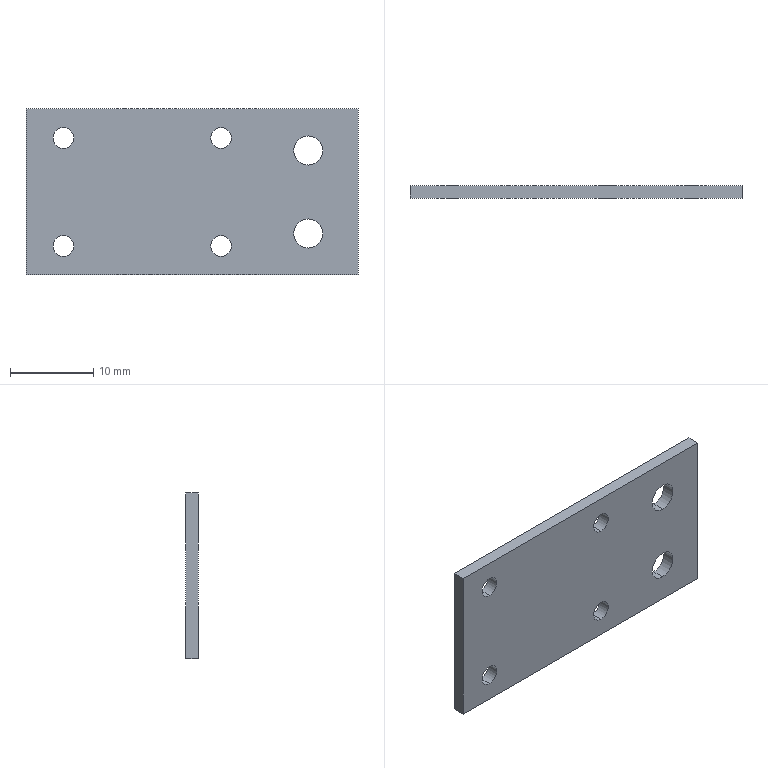Part | STEP file | 0243_224_Plate | 1 solid | 18 faces | box 40 x 1.5 x 20 mm | volume 1142 mm3 | cylinder 12 | plane 6 | commonest cylinder face diameters 2.5 x8 3.5 x4
STEP:
#1=CARTESIAN_POINT('',(0.,0.,0.));
#2=DIRECTION('',(0.,0.,1.));
#3=DIRECTION('',(1.,0.,0.));
#4=AXIS2_PLACEMENT_3D('',#1,#2,#3);
#5=CARTESIAN_POINT('',(-16.5,0.,7.75));
#6=VERTEX_POINT('',#5);
#7=CARTESIAN_POINT('',(-16.5,1.5,7.75));
#8=VERTEX_POINT('',#7);
#9=CARTESIAN_POINT('',(-16.5,1.5,7.75));
#10=DIRECTION('',(0.,1.,0.));
#11=VECTOR('',#10,1.);
#12=LINE('',#9,#11);
#13=CARTESIAN_POINT('',(-16.5,1.5,6.5));
#14=DIRECTION('',(0.,1.,0.));
#15=DIRECTION('',(0.,0.,1.));
#16=AXIS2_PLACEMENT_3D('',#13,#14,#15);
#17=CYLINDRICAL_SURFACE('',#16,1.25);
#18=CARTESIAN_POINT('',(6.283,0.));
#19=DIRECTION('',(0.,1.));
#20=VECTOR('',#19,1.);
#21=LINE('',#18,#20);
#22=(GEOMETRIC_REPRESENTATION_CONTEXT(2)PARAMETRIC_REPRESENTATION_CONTEXT()REPRESENTATION_CONTEXT('',''));
#23=DEFINITIONAL_REPRESENTATION('',(#21),#22);
#24=PCURVE('',#17,#23);
#25=CARTESIAN_POINT('',(-16.5,1.5,6.5));
#26=DIRECTION('',(0.,1.,0.));
#27=DIRECTION('',(0.,0.,1.));
#28=AXIS2_PLACEMENT_3D('',#25,#26,#27);
#29=CYLINDRICAL_SURFACE('',#28,1.25);
#30=CARTESIAN_POINT('',(0.,0.));
#31=DIRECTION('',(0.,1.));
#32=VECTOR('',#31,1.);
#33=LINE('',#30,#32);
#34=(GEOMETRIC_REPRESENTATION_CONTEXT(2)PARAMETRIC_REPRESENTATION_CONTEXT()REPRESENTATION_CONTEXT('',''));
#35=DEFINITIONAL_REPRESENTATION('',(#33),#34);
#36=PCURVE('',#29,#35);
#37=SURFACE_CURVE('',#12,(#24,#36),.PCURVE_S1.);
#38=EDGE_CURVE('',#6,#8,#37,.T.);
#39=ORIENTED_EDGE('',*,*,#38,.T.);
#40=CARTESIAN_POINT('',(-16.5,1.5,5.25));
#41=VERTEX_POINT('',#40);
#42=CARTESIAN_POINT('',(-16.5,1.5,6.5));
#43=DIRECTION('',(0.,1.,0.));
#44=DIRECTION('',(0.,0.,1.));
#45=AXIS2_PLACEMENT_3D('',#42,#43,#44);
#46=CIRCLE('',#45,1.25);
#47=CARTESIAN_POINT('',(0.,0.));
#48=DIRECTION('',(1.,0.));
#49=VECTOR('',#48,1.);
#50=LINE('',#47,#49);
#51=(GEOMETRIC_REPRESENTATION_CONTEXT(2)PARAMETRIC_REPRESENTATION_CONTEXT()REPRESENTATION_CONTEXT('',''));
#52=DEFINITIONAL_REPRESENTATION('',(#50),#51);
#53=PCURVE('',#17,#52);
#54=CARTESIAN_POINT('',(0.,1.5,-10.));
#55=DIRECTION('',(0.,1.,0.));
#56=DIRECTION('',(0.,0.,1.));
#57=AXIS2_PLACEMENT_3D('',#54,#55,#56);
#58=PLANE('',#57);
#59=CARTESIAN_POINT('',(16.5,-16.5));
#60=DIRECTION('',(1.,0.));
#61=AXIS2_PLACEMENT_2D('',#59,#60);
#62=CIRCLE('',#61,1.25);
#63=(GEOMETRIC_REPRESENTATION_CONTEXT(2)PARAMETRIC_REPRESENTATION_CONTEXT()REPRESENTATION_CONTEXT('',''));
#64=DEFINITIONAL_REPRESENTATION('',(#62),#63);
#65=PCURVE('',#58,#64);
#66=SURFACE_CURVE('',#46,(#53,#65),.PCURVE_S1.);
#67=EDGE_CURVE('',#41,#8,#66,.T.);
#68=ORIENTED_EDGE('',*,*,#67,.F.);
#69=CARTESIAN_POINT('',(-16.5,0.,5.25));
#70=VERTEX_POINT('',#69);
#71=CARTESIAN_POINT('',(-16.5,1.5,5.25));
#72=DIRECTION('',(0.,1.,0.));
#73=VECTOR('',#72,1.);
#74=LINE('',#71,#73);
#75=CARTESIAN_POINT('',(3.142,0.));
#76=DIRECTION('',(0.,1.));
#77=VECTOR('',#76,1.);
#78=LINE('',#75,#77);
#79=(GEOMETRIC_REPRESENTATION_CONTEXT(2)PARAMETRIC_REPRESENTATION_CONTEXT()REPRESENTATION_CONTEXT('',''));
#80=DEFINITIONAL_REPRESENTATION('',(#78),#79);
#81=PCURVE('',#17,#80);
#82=CARTESIAN_POINT('',(3.142,0.));
#83=DIRECTION('',(0.,1.));
#84=VECTOR('',#83,1.);
#85=LINE('',#82,#84);
#86=(GEOMETRIC_REPRESENTATION_CONTEXT(2)PARAMETRIC_REPRESENTATION_CONTEXT()REPRESENTATION_CONTEXT('',''));
#87=DEFINITIONAL_REPRESENTATION('',(#85),#86);
#88=PCURVE('',#29,#87);
#89=SURFACE_CURVE('',#74,(#81,#88),.PCURVE_S1.);
#90=EDGE_CURVE('',#70,#41,#89,.T.);
#91=ORIENTED_EDGE('',*,*,#90,.F.);
#92=CARTESIAN_POINT('',(-16.5,0.,6.5));
#93=DIRECTION('',(0.,1.,0.));
#94=DIRECTION('',(0.,0.,1.));
#95=AXIS2_PLACEMENT_3D('',#92,#93,#94);
#96=CIRCLE('',#95,1.25);
#97=CARTESIAN_POINT('',(0.,-1.5));
#98=DIRECTION('',(1.,0.));
#99=VECTOR('',#98,1.);
#100=LINE('',#97,#99);
#101=(GEOMETRIC_REPRESENTATION_CONTEXT(2)PARAMETRIC_REPRESENTATION_CONTEXT()REPRESENTATION_CONTEXT('',''));
#102=DEFINITIONAL_REPRESENTATION('',(#100),#101);
#103=PCURVE('',#17,#102);
#104=CARTESIAN_POINT('',(0.,0.,-10.));
#105=DIRECTION('',(0.,1.,0.));
#106=DIRECTION('',(0.,0.,1.));
#107=AXIS2_PLACEMENT_3D('',#104,#105,#106);
#108=PLANE('',#107);
#109=CARTESIAN_POINT('',(16.5,-16.5));
#110=DIRECTION('',(1.,0.));
#111=AXIS2_PLACEMENT_2D('',#109,#110);
#112=CIRCLE('',#111,1.25);
#113=(GEOMETRIC_REPRESENTATION_CONTEXT(2)PARAMETRIC_REPRESENTATION_CONTEXT()REPRESENTATION_CONTEXT('',''));
#114=DEFINITIONAL_REPRESENTATION('',(#112),#113);
#115=PCURVE('',#108,#114);
#116=SURFACE_CURVE('',#96,(#103,#115),.PCURVE_S1.);
#117=EDGE_CURVE('',#70,#6,#116,.T.);
#118=ORIENTED_EDGE('',*,*,#117,.T.);
#119=EDGE_LOOP('',(#39,#68,#91,#118));
#120=FACE_BOUND('',#119,.F.);
#121=ADVANCED_FACE('',(#120),#17,.F.);
#122=CARTESIAN_POINT('',(-16.5,0.,-5.25));
#123=VERTEX_POINT('',#122);
#124=CARTESIAN_POINT('',(-16.5,1.5,-5.25));
#125=VERTEX_POINT('',#124);
#126=CARTESIAN_POINT('',(-16.5,1.5,-5.25));
#127=DIRECTION('',(0.,1.,0.));
#128=VECTOR('',#127,1.);
#129=LINE('',#126,#128);
#130=CARTESIAN_POINT('',(-16.5,1.5,-6.5));
#131=DIRECTION('',(0.,1.,0.));
#132=DIRECTION('',(0.,0.,1.));
#133=AXIS2_PLACEMENT_3D('',#130,#131,#132);
#134=CYLINDRICAL_SURFACE('',#133,1.25);
#135=CARTESIAN_POINT('',(6.283,0.));
#136=DIRECTION('',(0.,1.));
#137=VECTOR('',#136,1.);
#138=LINE('',#135,#137);
#139=(GEOMETRIC_REPRESENTATION_CONTEXT(2)PARAMETRIC_REPRESENTATION_CONTEXT()REPRESENTATION_CONTEXT('',''));
#140=DEFINITIONAL_REPRESENTATION('',(#138),#139);
#141=PCURVE('',#134,#140);
#142=CARTESIAN_POINT('',(-16.5,1.5,-6.5));
#143=DIRECTION('',(0.,1.,0.));
#144=DIRECTION('',(0.,0.,1.));
#145=AXIS2_PLACEMENT_3D('',#142,#143,#144);
#146=CYLINDRICAL_SURFACE('',#145,1.25);
#147=CARTESIAN_POINT('',(0.,0.));
#148=DIRECTION('',(0.,1.));
#149=VECTOR('',#148,1.);
#150=LINE('',#147,#149);
#151=(GEOMETRIC_REPRESENTATION_CONTEXT(2)PARAMETRIC_REPRESENTATION_CONTEXT()REPRESENTATION_CONTEXT('',''));
#152=DEFINITIONAL_REPRESENTATION('',(#150),#151);
#153=PCURVE('',#146,#152);
#154=SURFACE_CURVE('',#129,(#141,#153),.PCURVE_S1.);
#155=EDGE_CURVE('',#123,#125,#154,.T.);
#156=ORIENTED_EDGE('',*,*,#155,.T.);
#157=CARTESIAN_POINT('',(-16.5,1.5,-7.75));
#158=VERTEX_POINT('',#157);
#159=CARTESIAN_POINT('',(-16.5,1.5,-6.5));
#160=DIRECTION('',(0.,1.,0.));
#161=DIRECTION('',(0.,0.,1.));
#162=AXIS2_PLACEMENT_3D('',#159,#160,#161);
#163=CIRCLE('',#162,1.25);
#164=CARTESIAN_POINT('',(0.,0.));
#165=DIRECTION('',(1.,0.));
#166=VECTOR('',#165,1.);
#167=LINE('',#164,#166);
#168=(GEOMETRIC_REPRESENTATION_CONTEXT(2)PARAMETRIC_REPRESENTATION_CONTEXT()REPRESENTATION_CONTEXT('',''));
#169=DEFINITIONAL_REPRESENTATION('',(#167),#168);
#170=PCURVE('',#134,#169);
#171=CARTESIAN_POINT('',(3.5,-16.5));
#172=DIRECTION('',(1.,0.));
#173=AXIS2_PLACEMENT_2D('',#171,#172);
#174=CIRCLE('',#173,1.25);
#175=(GEOMETRIC_REPRESENTATION_CONTEXT(2)PARAMETRIC_REPRESENTATION_CONTEXT()REPRESENTATION_CONTEXT('',''));
#176=DEFINITIONAL_REPRESENTATION('',(#174),#175);
#177=PCURVE('',#58,#176);
#178=SURFACE_CURVE('',#163,(#170,#177),.PCURVE_S1.);
#179=EDGE_CURVE('',#158,#125,#178,.T.);
#180=ORIENTED_EDGE('',*,*,#179,.F.);
#181=CARTESIAN_POINT('',(-16.5,0.,-7.75));
#182=VERTEX_POINT('',#181);
#183=CARTESIAN_POINT('',(-16.5,1.5,-7.75));
#184=DIRECTION('',(0.,1.,0.));
#185=VECTOR('',#184,1.);
#186=LINE('',#183,#185);
#187=CARTESIAN_POINT('',(3.142,0.));
#188=DIRECTION('',(0.,1.));
#189=VECTOR('',#188,1.);
#190=LINE('',#187,#189);
#191=(GEOMETRIC_REPRESENTATION_CONTEXT(2)PARAMETRIC_REPRESENTATION_CONTEXT()REPRESENTATION_CONTEXT('',''));
#192=DEFINITIONAL_REPRESENTATION('',(#190),#191);
#193=PCURVE('',#134,#192);
#194=CARTESIAN_POINT('',(3.142,0.));
#195=DIRECTION('',(0.,1.));
#196=VECTOR('',#195,1.);
#197=LINE('',#194,#196);
#198=(GEOMETRIC_REPRESENTATION_CONTEXT(2)PARAMETRIC_REPRESENTATION_CONTEXT()REPRESENTATION_CONTEXT('',''));
#199=DEFINITIONAL_REPRESENTATION('',(#197),#198);
#200=PCURVE('',#146,#199);
#201=SURFACE_CURVE('',#186,(#193,#200),.PCURVE_S1.);
#202=EDGE_CURVE('',#182,#158,#201,.T.);
#203=ORIENTED_EDGE('',*,*,#202,.F.);
#204=CARTESIAN_POINT('',(-16.5,0.,-6.5));
#205=DIRECTION('',(0.,1.,0.));
#206=DIRECTION('',(0.,0.,1.));
#207=AXIS2_PLACEMENT_3D('',#204,#205,#206);
#208=CIRCLE('',#207,1.25);
#209=CARTESIAN_POINT('',(0.,-1.5));
#210=DIRECTION('',(1.,0.));
#211=VECTOR('',#210,1.);
#212=LINE('',#209,#211);
#213=(GEOMETRIC_REPRESENTATION_CONTEXT(2)PARAMETRIC_REPRESENTATION_CONTEXT()REPRESENTATION_CONTEXT('',''));
#214=DEFINITIONAL_REPRESENTATION('',(#212),#213);
#215=PCURVE('',#134,#214);
#216=CARTESIAN_POINT('',(3.5,-16.5));
#217=DIRECTION('',(1.,0.));
#218=AXIS2_PLACEMENT_2D('',#216,#217);
#219=CIRCLE('',#218,1.25);
#220=(GEOMETRIC_REPRESENTATION_CONTEXT(2)PARAMETRIC_REPRESENTATION_CONTEXT()REPRESENTATION_CONTEXT('',''));
#221=DEFINITIONAL_REPRESENTATION('',(#219),#220);
#222=PCURVE('',#108,#221);
#223=SURFACE_CURVE('',#208,(#215,#222),.PCURVE_S1.);
#224=EDGE_CURVE('',#182,#123,#223,.T.);
#225=ORIENTED_EDGE('',*,*,#224,.T.);
#226=EDGE_LOOP('',(#156,#180,#203,#225));
#227=FACE_BOUND('',#226,.F.);
#228=ADVANCED_FACE('',(#227),#134,.F.);
#229=CARTESIAN_POINT('',(-35.5,0.,-5.25));
#230=VERTEX_POINT('',#229);
#231=CARTESIAN_POINT('',(-35.5,1.5,-5.25));
#232=VERTEX_POINT('',#231);
#233=CARTESIAN_POINT('',(-35.5,1.5,-5.25));
#234=DIRECTION('',(0.,1.,0.));
#235=VECTOR('',#234,1.);
#236=LINE('',#233,#235);
#237=CARTESIAN_POINT('',(-35.5,1.5,-6.5));
#238=DIRECTION('',(0.,1.,0.));
#239=DIRECTION('',(0.,0.,1.));
#240=AXIS2_PLACEMENT_3D('',#237,#238,#239);
#241=CYLINDRICAL_SURFACE('',#240,1.25);
#242=CARTESIAN_POINT('',(6.283,0.));
#243=DIRECTION('',(0.,1.));
#244=VECTOR('',#243,1.);
#245=LINE('',#242,#244);
#246=(GEOMETRIC_REPRESENTATION_CONTEXT(2)PARAMETRIC_REPRESENTATION_CONTEXT()REPRESENTATION_CONTEXT('',''));
#247=DEFINITIONAL_REPRESENTATION('',(#245),#246);
#248=PCURVE('',#241,#247);
#249=CARTESIAN_POINT('',(-35.5,1.5,-6.5));
#250=DIRECTION('',(0.,1.,0.));
#251=DIRECTION('',(0.,0.,1.));
#252=AXIS2_PLACEMENT_3D('',#249,#250,#251);
#253=CYLINDRICAL_SURFACE('',#252,1.25);
#254=CARTESIAN_POINT('',(0.,0.));
#255=DIRECTION('',(0.,1.));
#256=VECTOR('',#255,1.);
#257=LINE('',#254,#256);
#258=(GEOMETRIC_REPRESENTATION_CONTEXT(2)PARAMETRIC_REPRESENTATION_CONTEXT()REPRESENTATION_CONTEXT('',''));
#259=DEFINITIONAL_REPRESENTATION('',(#257),#258);
#260=PCURVE('',#253,#259);
#261=SURFACE_CURVE('',#236,(#248,#260),.PCURVE_S1.);
#262=EDGE_CURVE('',#230,#232,#261,.T.);
#263=ORIENTED_EDGE('',*,*,#262,.T.);
#264=CARTESIAN_POINT('',(-35.5,1.5,-7.75));
#265=VERTEX_POINT('',#264);
#266=CARTESIAN_POINT('',(-35.5,1.5,-6.5));
#267=DIRECTION('',(0.,1.,0.));
#268=DIRECTION('',(0.,0.,1.));
#269=AXIS2_PLACEMENT_3D('',#266,#267,#268);
#270=CIRCLE('',#269,1.25);
#271=CARTESIAN_POINT('',(0.,0.));
#272=DIRECTION('',(1.,0.));
#273=VECTOR('',#272,1.);
#274=LINE('',#271,#273);
#275=(GEOMETRIC_REPRESENTATION_CONTEXT(2)PARAMETRIC_REPRESENTATION_CONTEXT()REPRESENTATION_CONTEXT('',''));
#276=DEFINITIONAL_REPRESENTATION('',(#274),#275);
#277=PCURVE('',#241,#276);
#278=CARTESIAN_POINT('',(3.5,-35.5));
#279=DIRECTION('',(1.,0.));
#280=AXIS2_PLACEMENT_2D('',#278,#279);
#281=CIRCLE('',#280,1.25);
#282=(GEOMETRIC_REPRESENTATION_CONTEXT(2)PARAMETRIC_REPRESENTATION_CONTEXT()REPRESENTATION_CONTEXT('',''));
#283=DEFINITIONAL_REPRESENTATION('',(#281),#282);
#284=PCURVE('',#58,#283);
#285=SURFACE_CURVE('',#270,(#277,#284),.PCURVE_S1.);
#286=EDGE_CURVE('',#265,#232,#285,.T.);
#287=ORIENTED_EDGE('',*,*,#286,.F.);
#288=CARTESIAN_POINT('',(-35.5,0.,-7.75));
#289=VERTEX_POINT('',#288);
#290=CARTESIAN_POINT('',(-35.5,1.5,-7.75));
#291=DIRECTION('',(0.,1.,0.));
#292=VECTOR('',#291,1.);
#293=LINE('',#290,#292);
#294=CARTESIAN_POINT('',(3.142,0.));
#295=DIRECTION('',(0.,1.));
#296=VECTOR('',#295,1.);
#297=LINE('',#294,#296);
#298=(GEOMETRIC_REPRESENTATION_CONTEXT(2)PARAMETRIC_REPRESENTATION_CONTEXT()REPRESENTATION_CONTEXT('',''));
#299=DEFINITIONAL_REPRESENTATION('',(#297),#298);
#300=PCURVE('',#241,#299);
#301=CARTESIAN_POINT('',(3.142,0.));
#302=DIRECTION('',(0.,1.));
#303=VECTOR('',#302,1.);
#304=LINE('',#301,#303);
#305=(GEOMETRIC_REPRESENTATION_CONTEXT(2)PARAMETRIC_REPRESENTATION_CONTEXT()REPRESENTATION_CONTEXT('',''));
#306=DEFINITIONAL_REPRESENTATION('',(#304),#305);
#307=PCURVE('',#253,#306);
#308=SURFACE_CURVE('',#293,(#300,#307),.PCURVE_S1.);
#309=EDGE_CURVE('',#289,#265,#308,.T.);
#310=ORIENTED_EDGE('',*,*,#309,.F.);
#311=CARTESIAN_POINT('',(-35.5,0.,-6.5));
#312=DIRECTION('',(0.,1.,0.));
#313=DIRECTION('',(0.,0.,1.));
#314=AXIS2_PLACEMENT_3D('',#311,#312,#313);
#315=CIRCLE('',#314,1.25);
#316=CARTESIAN_POINT('',(0.,-1.5));
#317=DIRECTION('',(1.,0.));
#318=VECTOR('',#317,1.);
#319=LINE('',#316,#318);
#320=(GEOMETRIC_REPRESENTATION_CONTEXT(2)PARAMETRIC_REPRESENTATION_CONTEXT()REPRESENTATION_CONTEXT('',''));
#321=DEFINITIONAL_REPRESENTATION('',(#319),#320);
#322=PCURVE('',#241,#321);
#323=CARTESIAN_POINT('',(3.5,-35.5));
#324=DIRECTION('',(1.,0.));
#325=AXIS2_PLACEMENT_2D('',#323,#324);
#326=CIRCLE('',#325,1.25);
#327=(GEOMETRIC_REPRESENTATION_CONTEXT(2)PARAMETRIC_REPRESENTATION_CONTEXT()REPRESENTATION_CONTEXT('',''));
#328=DEFINITIONAL_REPRESENTATION('',(#326),#327);
#329=PCURVE('',#108,#328);
#330=SURFACE_CURVE('',#315,(#322,#329),.PCURVE_S1.);
#331=EDGE_CURVE('',#289,#230,#330,.T.);
#332=ORIENTED_EDGE('',*,*,#331,.T.);
#333=EDGE_LOOP('',(#263,#287,#310,#332));
#334=FACE_BOUND('',#333,.F.);
#335=ADVANCED_FACE('',(#334),#241,.F.);
#336=CARTESIAN_POINT('',(-35.5,0.,7.75));
#337=VERTEX_POINT('',#336);
#338=CARTESIAN_POINT('',(-35.5,1.5,7.75));
#339=VERTEX_POINT('',#338);
#340=CARTESIAN_POINT('',(-35.5,1.5,7.75));
#341=DIRECTION('',(0.,1.,0.));
#342=VECTOR('',#341,1.);
#343=LINE('',#340,#342);
#344=CARTESIAN_POINT('',(-35.5,1.5,6.5));
#345=DIRECTION('',(0.,1.,0.));
#346=DIRECTION('',(0.,0.,1.));
#347=AXIS2_PLACEMENT_3D('',#344,#345,#346);
#348=CYLINDRICAL_SURFACE('',#347,1.25);
#349=CARTESIAN_POINT('',(6.283,0.));
#350=DIRECTION('',(0.,1.));
#351=VECTOR('',#350,1.);
#352=LINE('',#349,#351);
#353=(GEOMETRIC_REPRESENTATION_CONTEXT(2)PARAMETRIC_REPRESENTATION_CONTEXT()REPRESENTATION_CONTEXT('',''));
#354=DEFINITIONAL_REPRESENTATION('',(#352),#353);
#355=PCURVE('',#348,#354);
#356=CARTESIAN_POINT('',(-35.5,1.5,6.5));
#357=DIRECTION('',(0.,1.,0.));
#358=DIRECTION('',(0.,0.,1.));
#359=AXIS2_PLACEMENT_3D('',#356,#357,#358);
#360=CYLINDRICAL_SURFACE('',#359,1.25);
#361=CARTESIAN_POINT('',(0.,0.));
#362=DIRECTION('',(0.,1.));
#363=VECTOR('',#362,1.);
#364=LINE('',#361,#363);
#365=(GEOMETRIC_REPRESENTATION_CONTEXT(2)PARAMETRIC_REPRESENTATION_CONTEXT()REPRESENTATION_CONTEXT('',''));
#366=DEFINITIONAL_REPRESENTATION('',(#364),#365);
#367=PCURVE('',#360,#366);
#368=SURFACE_CURVE('',#343,(#355,#367),.PCURVE_S1.);
#369=EDGE_CURVE('',#337,#339,#368,.T.);
#370=ORIENTED_EDGE('',*,*,#369,.T.);
#371=CARTESIAN_POINT('',(-35.5,1.5,5.25));
#372=VERTEX_POINT('',#371);
#373=CARTESIAN_POINT('',(-35.5,1.5,6.5));
#374=DIRECTION('',(0.,1.,0.));
#375=DIRECTION('',(0.,0.,1.));
#376=AXIS2_PLACEMENT_3D('',#373,#374,#375);
#377=CIRCLE('',#376,1.25);
#378=CARTESIAN_POINT('',(0.,0.));
#379=DIRECTION('',(1.,0.));
#380=VECTOR('',#379,1.);
#381=LINE('',#378,#380);
#382=(GEOMETRIC_REPRESENTATION_CONTEXT(2)PARAMETRIC_REPRESENTATION_CONTEXT()REPRESENTATION_CONTEXT('',''));
#383=DEFINITIONAL_REPRESENTATION('',(#381),#382);
#384=PCURVE('',#348,#383);
#385=CARTESIAN_POINT('',(16.5,-35.5));
#386=DIRECTION('',(1.,0.));
#387=AXIS2_PLACEMENT_2D('',#385,#386);
#388=CIRCLE('',#387,1.25);
#389=(GEOMETRIC_REPRESENTATION_CONTEXT(2)PARAMETRIC_REPRESENTATION_CONTEXT()REPRESENTATION_CONTEXT('',''));
#390=DEFINITIONAL_REPRESENTATION('',(#388),#389);
#391=PCURVE('',#58,#390);
#392=SURFACE_CURVE('',#377,(#384,#391),.PCURVE_S1.);
#393=EDGE_CURVE('',#372,#339,#392,.T.);
#394=ORIENTED_EDGE('',*,*,#393,.F.);
#395=CARTESIAN_POINT('',(-35.5,0.,5.25));
#396=VERTEX_POINT('',#395);
#397=CARTESIAN_POINT('',(-35.5,1.5,5.25));
#398=DIRECTION('',(0.,1.,0.));
#399=VECTOR('',#398,1.);
#400=LINE('',#397,#399);
#401=CARTESIAN_POINT('',(3.142,0.));
#402=DIRECTION('',(0.,1.));
#403=VECTOR('',#402,1.);
#404=LINE('',#401,#403);
#405=(GEOMETRIC_REPRESENTATION_CONTEXT(2)PARAMETRIC_REPRESENTATION_CONTEXT()REPRESENTATION_CONTEXT('',''));
#406=DEFINITIONAL_REPRESENTATION('',(#404),#405);
#407=PCURVE('',#348,#406);
#408=CARTESIAN_POINT('',(3.142,0.));
#409=DIRECTION('',(0.,1.));
#410=VECTOR('',#409,1.);
#411=LINE('',#408,#410);
#412=(GEOMETRIC_REPRESENTATION_CONTEXT(2)PARAMETRIC_REPRESENTATION_CONTEXT()REPRESENTATION_CONTEXT('',''));
#413=DEFINITIONAL_REPRESENTATION('',(#411),#412);
#414=PCURVE('',#360,#413);
#415=SURFACE_CURVE('',#400,(#407,#414),.PCURVE_S1.);
#416=EDGE_CURVE('',#396,#372,#415,.T.);
#417=ORIENTED_EDGE('',*,*,#416,.F.);
#418=CARTESIAN_POINT('',(-35.5,0.,6.5));
#419=DIRECTION('',(0.,1.,0.));
#420=DIRECTION('',(0.,0.,1.));
#421=AXIS2_PLACEMENT_3D('',#418,#419,#420);
#422=CIRCLE('',#421,1.25);
#423=CARTESIAN_POINT('',(0.,-1.5));
#424=DIRECTION('',(1.,0.));
#425=VECTOR('',#424,1.);
#426=LINE('',#423,#425);
#427=(GEOMETRIC_REPRESENTATION_CONTEXT(2)PARAMETRIC_REPRESENTATION_CONTEXT()REPRESENTATION_CONTEXT('',''));
#428=DEFINITIONAL_REPRESENTATION('',(#426),#427);
#429=PCURVE('',#348,#428);
#430=CARTESIAN_POINT('',(16.5,-35.5));
#431=DIRECTION('',(1.,0.));
#432=AXIS2_PLACEMENT_2D('',#430,#431);
#433=CIRCLE('',#432,1.25);
#434=(GEOMETRIC_REPRESENTATION_CONTEXT(2)PARAMETRIC_REPRESENTATION_CONTEXT()REPRESENTATION_CONTEXT('',''));
#435=DEFINITIONAL_REPRESENTATION('',(#433),#434);
#436=PCURVE('',#108,#435);
#437=SURFACE_CURVE('',#422,(#429,#436),.PCURVE_S1.);
#438=EDGE_CURVE('',#396,#337,#437,.T.);
#439=ORIENTED_EDGE('',*,*,#438,.T.);
#440=EDGE_LOOP('',(#370,#394,#417,#439));
#441=FACE_BOUND('',#440,.F.);
#442=ADVANCED_FACE('',(#441),#348,.F.);
#443=CARTESIAN_POINT('',(-6.,0.,6.75));
#444=VERTEX_POINT('',#443);
#445=CARTESIAN_POINT('',(-6.,1.5,6.75));
#446=VERTEX_POINT('',#445);
#447=CARTESIAN_POINT('',(-6.,1.5,6.75));
#448=DIRECTION('',(0.,1.,0.));
#449=VECTOR('',#448,1.);
#450=LINE('',#447,#449);
#451=CARTESIAN_POINT('',(-6.,1.5,5.));
#452=DIRECTION('',(0.,1.,0.));
#453=DIRECTION('',(0.,0.,1.));
#454=AXIS2_PLACEMENT_3D('',#451,#452,#453);
#455=CYLINDRICAL_SURFACE('',#454,1.75);
#456=CARTESIAN_POINT('',(6.283,0.));
#457=DIRECTION('',(0.,1.));
#458=VECTOR('',#457,1.);
#459=LINE('',#456,#458);
#460=(GEOMETRIC_REPRESENTATION_CONTEXT(2)PARAMETRIC_REPRESENTATION_CONTEXT()REPRESENTATION_CONTEXT('',''));
#461=DEFINITIONAL_REPRESENTATION('',(#459),#460);
#462=PCURVE('',#455,#461);
#463=CARTESIAN_POINT('',(-6.,1.5,5.));
#464=DIRECTION('',(0.,1.,0.));
#465=DIRECTION('',(0.,0.,1.));
#466=AXIS2_PLACEMENT_3D('',#463,#464,#465);
#467=CYLINDRICAL_SURFACE('',#466,1.75);
#468=CARTESIAN_POINT('',(0.,0.));
#469=DIRECTION('',(0.,1.));
#470=VECTOR('',#469,1.);
#471=LINE('',#468,#470);
#472=(GEOMETRIC_REPRESENTATION_CONTEXT(2)PARAMETRIC_REPRESENTATION_CONTEXT()REPRESENTATION_CONTEXT('',''));
#473=DEFINITIONAL_REPRESENTATION('',(#471),#472);
#474=PCURVE('',#467,#473);
#475=SURFACE_CURVE('',#450,(#462,#474),.PCURVE_S1.);
#476=EDGE_CURVE('',#444,#446,#475,.T.);
#477=ORIENTED_EDGE('',*,*,#476,.T.);
#478=CARTESIAN_POINT('',(-6.,1.5,3.25));
#479=VERTEX_POINT('',#478);
#480=CARTESIAN_POINT('',(-6.,1.5,5.));
#481=DIRECTION('',(0.,1.,0.));
#482=DIRECTION('',(0.,0.,1.));
#483=AXIS2_PLACEMENT_3D('',#480,#481,#482);
#484=CIRCLE('',#483,1.75);
#485=CARTESIAN_POINT('',(0.,0.));
#486=DIRECTION('',(1.,0.));
#487=VECTOR('',#486,1.);
#488=LINE('',#485,#487);
#489=(GEOMETRIC_REPRESENTATION_CONTEXT(2)PARAMETRIC_REPRESENTATION_CONTEXT()REPRESENTATION_CONTEXT('',''));
#490=DEFINITIONAL_REPRESENTATION('',(#488),#489);
#491=PCURVE('',#455,#490);
#492=CARTESIAN_POINT('',(15.,-6.));
#493=DIRECTION('',(1.,0.));
#494=AXIS2_PLACEMENT_2D('',#492,#493);
#495=CIRCLE('',#494,1.75);
#496=(GEOMETRIC_REPRESENTATION_CONTEXT(2)PARAMETRIC_REPRESENTATION_CONTEXT()REPRESENTATION_CONTEXT('',''));
#497=DEFINITIONAL_REPRESENTATION('',(#495),#496);
#498=PCURVE('',#58,#497);
#499=SURFACE_CURVE('',#484,(#491,#498),.PCURVE_S1.);
#500=EDGE_CURVE('',#479,#446,#499,.T.);
#501=ORIENTED_EDGE('',*,*,#500,.F.);
#502=CARTESIAN_POINT('',(-6.,0.,3.25));
#503=VERTEX_POINT('',#502);
#504=CARTESIAN_POINT('',(-6.,1.5,3.25));
#505=DIRECTION('',(0.,1.,0.));
#506=VECTOR('',#505,1.);
#507=LINE('',#504,#506);
#508=CARTESIAN_POINT('',(3.142,0.));
#509=DIRECTION('',(0.,1.));
#510=VECTOR('',#509,1.);
#511=LINE('',#508,#510);
#512=(GEOMETRIC_REPRESENTATION_CONTEXT(2)PARAMETRIC_REPRESENTATION_CONTEXT()REPRESENTATION_CONTEXT('',''));
#513=DEFINITIONAL_REPRESENTATION('',(#511),#512);
#514=PCURVE('',#455,#513);
#515=CARTESIAN_POINT('',(3.142,0.));
#516=DIRECTION('',(0.,1.));
#517=VECTOR('',#516,1.);
#518=LINE('',#515,#517);
#519=(GEOMETRIC_REPRESENTATION_CONTEXT(2)PARAMETRIC_REPRESENTATION_CONTEXT()REPRESENTATION_CONTEXT('',''));
#520=DEFINITIONAL_REPRESENTATION('',(#518),#519);
#521=PCURVE('',#467,#520);
#522=SURFACE_CURVE('',#507,(#514,#521),.PCURVE_S1.);
#523=EDGE_CURVE('',#503,#479,#522,.T.);
#524=ORIENTED_EDGE('',*,*,#523,.F.);
#525=CARTESIAN_POINT('',(-6.,0.,5.));
#526=DIRECTION('',(0.,1.,0.));
#527=DIRECTION('',(0.,0.,1.));
#528=AXIS2_PLACEMENT_3D('',#525,#526,#527);
#529=CIRCLE('',#528,1.75);
#530=CARTESIAN_POINT('',(0.,-1.5));
#531=DIRECTION('',(1.,0.));
#532=VECTOR('',#531,1.);
#533=LINE('',#530,#532);
#534=(GEOMETRIC_REPRESENTATION_CONTEXT(2)PARAMETRIC_REPRESENTATION_CONTEXT()REPRESENTATION_CONTEXT('',''));
#535=DEFINITIONAL_REPRESENTATION('',(#533),#534);
#536=PCURVE('',#455,#535);
#537=CARTESIAN_POINT('',(15.,-6.));
#538=DIRECTION('',(1.,0.));
#539=AXIS2_PLACEMENT_2D('',#537,#538);
#540=CIRCLE('',#539,1.75);
#541=(GEOMETRIC_REPRESENTATION_CONTEXT(2)PARAMETRIC_REPRESENTATION_CONTEXT()REPRESENTATION_CONTEXT('',''));
#542=DEFINITIONAL_REPRESENTATION('',(#540),#541);
#543=PCURVE('',#108,#542);
#544=SURFACE_CURVE('',#529,(#536,#543),.PCURVE_S1.);
#545=EDGE_CURVE('',#503,#444,#544,.T.);
#546=ORIENTED_EDGE('',*,*,#545,.T.);
#547=EDGE_LOOP('',(#477,#501,#524,#546));
#548=FACE_BOUND('',#547,.F.);
#549=ADVANCED_FACE('',(#548),#455,.F.);
#550=CARTESIAN_POINT('',(-6.,0.,-3.25));
#551=VERTEX_POINT('',#550);
#552=CARTESIAN_POINT('',(-6.,1.5,-3.25));
#553=VERTEX_POINT('',#552);
#554=CARTESIAN_POINT('',(-6.,1.5,-3.25));
#555=DIRECTION('',(0.,1.,0.));
#556=VECTOR('',#555,1.);
#557=LINE('',#554,#556);
#558=CARTESIAN_POINT('',(-6.,1.5,-5.));
#559=DIRECTION('',(0.,1.,0.));
#560=DIRECTION('',(0.,0.,1.));
#561=AXIS2_PLACEMENT_3D('',#558,#559,#560);
#562=CYLINDRICAL_SURFACE('',#561,1.75);
#563=CARTESIAN_POINT('',(6.283,0.));
#564=DIRECTION('',(0.,1.));
#565=VECTOR('',#564,1.);
#566=LINE('',#563,#565);
#567=(GEOMETRIC_REPRESENTATION_CONTEXT(2)PARAMETRIC_REPRESENTATION_CONTEXT()REPRESENTATION_CONTEXT('',''));
#568=DEFINITIONAL_REPRESENTATION('',(#566),#567);
#569=PCURVE('',#562,#568);
#570=CARTESIAN_POINT('',(-6.,1.5,-5.));
#571=DIRECTION('',(0.,1.,0.));
#572=DIRECTION('',(0.,0.,1.));
#573=AXIS2_PLACEMENT_3D('',#570,#571,#572);
#574=CYLINDRICAL_SURFACE('',#573,1.75);
#575=CARTESIAN_POINT('',(0.,0.));
#576=DIRECTION('',(0.,1.));
#577=VECTOR('',#576,1.);
#578=LINE('',#575,#577);
#579=(GEOMETRIC_REPRESENTATION_CONTEXT(2)PARAMETRIC_REPRESENTATION_CONTEXT()REPRESENTATION_CONTEXT('',''));
#580=DEFINITIONAL_REPRESENTATION('',(#578),#579);
#581=PCURVE('',#574,#580);
#582=SURFACE_CURVE('',#557,(#569,#581),.PCURVE_S1.);
#583=EDGE_CURVE('',#551,#553,#582,.T.);
#584=ORIENTED_EDGE('',*,*,#583,.T.);
#585=CARTESIAN_POINT('',(-6.,1.5,-6.75));
#586=VERTEX_POINT('',#585);
#587=CARTESIAN_POINT('',(-6.,1.5,-5.));
#588=DIRECTION('',(0.,1.,0.));
#589=DIRECTION('',(0.,0.,1.));
#590=AXIS2_PLACEMENT_3D('',#587,#588,#589);
#591=CIRCLE('',#590,1.75);
#592=CARTESIAN_POINT('',(0.,0.));
#593=DIRECTION('',(1.,0.));
#594=VECTOR('',#593,1.);
#595=LINE('',#592,#594);
#596=(GEOMETRIC_REPRESENTATION_CONTEXT(2)PARAMETRIC_REPRESENTATION_CONTEXT()REPRESENTATION_CONTEXT('',''));
#597=DEFINITIONAL_REPRESENTATION('',(#595),#596);
#598=PCURVE('',#562,#597);
#599=CARTESIAN_POINT('',(5.,-6.));
#600=DIRECTION('',(1.,0.));
#601=AXIS2_PLACEMENT_2D('',#599,#600);
#602=CIRCLE('',#601,1.75);
#603=(GEOMETRIC_REPRESENTATION_CONTEXT(2)PARAMETRIC_REPRESENTATION_CONTEXT()REPRESENTATION_CONTEXT('',''));
#604=DEFINITIONAL_REPRESENTATION('',(#602),#603);
#605=PCURVE('',#58,#604);
#606=SURFACE_CURVE('',#591,(#598,#605),.PCURVE_S1.);
#607=EDGE_CURVE('',#586,#553,#606,.T.);
#608=ORIENTED_EDGE('',*,*,#607,.F.);
#609=CARTESIAN_POINT('',(-6.,0.,-6.75));
#610=VERTEX_POINT('',#609);
#611=CARTESIAN_POINT('',(-6.,1.5,-6.75));
#612=DIRECTION('',(0.,1.,0.));
#613=VECTOR('',#612,1.);
#614=LINE('',#611,#613);
#615=CARTESIAN_POINT('',(3.142,0.));
#616=DIRECTION('',(0.,1.));
#617=VECTOR('',#616,1.);
#618=LINE('',#615,#617);
#619=(GEOMETRIC_REPRESENTATION_CONTEXT(2)PARAMETRIC_REPRESENTATION_CONTEXT()REPRESENTATION_CONTEXT('',''));
#620=DEFINITIONAL_REPRESENTATION('',(#618),#619);
#621=PCURVE('',#562,#620);
#622=CARTESIAN_POINT('',(3.142,0.));
#623=DIRECTION('',(0.,1.));
#624=VECTOR('',#623,1.);
#625=LINE('',#622,#624);
#626=(GEOMETRIC_REPRESENTATION_CONTEXT(2)PARAMETRIC_REPRESENTATION_CONTEXT()REPRESENTATION_CONTEXT('',''));
#627=DEFINITIONAL_REPRESENTATION('',(#625),#626);
#628=PCURVE('',#574,#627);
#629=SURFACE_CURVE('',#614,(#621,#628),.PCURVE_S1.);
#630=EDGE_CURVE('',#610,#586,#629,.T.);
#631=ORIENTED_EDGE('',*,*,#630,.F.);
#632=CARTESIAN_POINT('',(-6.,0.,-5.));
#633=DIRECTION('',(0.,1.,0.));
#634=DIRECTION('',(0.,0.,1.));
#635=AXIS2_PLACEMENT_3D('',#632,#633,#634);
#636=CIRCLE('',#635,1.75);
#637=CARTESIAN_POINT('',(0.,-1.5));
#638=DIRECTION('',(1.,0.));
#639=VECTOR('',#638,1.);
#640=LINE('',#637,#639);
#641=(GEOMETRIC_REPRESENTATION_CONTEXT(2)PARAMETRIC_REPRESENTATION_CONTEXT()REPRESENTATION_CONTEXT('',''));
#642=DEFINITIONAL_REPRESENTATION('',(#640),#641);
#643=PCURVE('',#562,#642);
#644=CARTESIAN_POINT('',(5.,-6.));
#645=DIRECTION('',(1.,0.));
#646=AXIS2_PLACEMENT_2D('',#644,#645);
#647=CIRCLE('',#646,1.75);
#648=(GEOMETRIC_REPRESENTATION_CONTEXT(2)PARAMETRIC_REPRESENTATION_CONTEXT()REPRESENTATION_CONTEXT('',''));
#649=DEFINITIONAL_REPRESENTATION('',(#647),#648);
#650=PCURVE('',#108,#649);
#651=SURFACE_CURVE('',#636,(#643,#650),.PCURVE_S1.);
#652=EDGE_CURVE('',#610,#551,#651,.T.);
#653=ORIENTED_EDGE('',*,*,#652,.T.);
#654=EDGE_LOOP('',(#584,#608,#631,#653));
#655=FACE_BOUND('',#654,.F.);
#656=ADVANCED_FACE('',(#655),#562,.F.);
#657=CARTESIAN_POINT('',(0.,0.,10.));
#658=VERTEX_POINT('',#657);
#659=CARTESIAN_POINT('',(0.,0.,-10.));
#660=VERTEX_POINT('',#659);
#661=CARTESIAN_POINT('',(0.,0.,10.));
#662=DIRECTION('',(0.,0.,-1.));
#663=VECTOR('',#662,1.);
#664=LINE('',#661,#663);
#665=CARTESIAN_POINT('',(0.,1.5,10.));
#666=DIRECTION('',(-1.,0.,0.));
#667=DIRECTION('',(0.,0.,1.));
#668=AXIS2_PLACEMENT_3D('',#665,#666,#667);
#669=PLANE('',#668);
#670=CARTESIAN_POINT('',(0.,-1.5));
#671=DIRECTION('',(-1.,0.));
#672=VECTOR('',#671,1.);
#673=LINE('',#670,#672);
#674=(GEOMETRIC_REPRESENTATION_CONTEXT(2)PARAMETRIC_REPRESENTATION_CONTEXT()REPRESENTATION_CONTEXT('',''));
#675=DEFINITIONAL_REPRESENTATION('',(#673),#674);
#676=PCURVE('',#669,#675);
#677=CARTESIAN_POINT('',(20.,0.));
#678=DIRECTION('',(-1.,0.));
#679=VECTOR('',#678,1.);
#680=LINE('',#677,#679);
#681=(GEOMETRIC_REPRESENTATION_CONTEXT(2)PARAMETRIC_REPRESENTATION_CONTEXT()REPRESENTATION_CONTEXT('',''));
#682=DEFINITIONAL_REPRESENTATION('',(#680),#681);
#683=PCURVE('',#108,#682);
#684=SURFACE_CURVE('',#664,(#676,#683),.PCURVE_S1.);
#685=EDGE_CURVE('',#658,#660,#684,.T.);
#686=ORIENTED_EDGE('',*,*,#685,.T.);
#687=CARTESIAN_POINT('',(0.,1.5,-10.));
#688=VERTEX_POINT('',#687);
#689=CARTESIAN_POINT('',(0.,1.5,-10.));
#690=DIRECTION('',(0.,-1.,0.));
#691=VECTOR('',#690,1.);
#692=LINE('',#689,#691);
#693=CARTESIAN_POINT('',(-20.,0.));
#694=DIRECTION('',(0.,-1.));
#695=VECTOR('',#694,1.);
#696=LINE('',#693,#695);
#697=(GEOMETRIC_REPRESENTATION_CONTEXT(2)PARAMETRIC_REPRESENTATION_CONTEXT()REPRESENTATION_CONTEXT('',''));
#698=DEFINITIONAL_REPRESENTATION('',(#696),#697);
#699=PCURVE('',#669,#698);
#700=CARTESIAN_POINT('',(0.,1.5,-10.));
#701=DIRECTION('',(0.,0.,1.));
#702=DIRECTION('',(1.,0.,0.));
#703=AXIS2_PLACEMENT_3D('',#700,#701,#702);
#704=PLANE('',#703);
#705=CARTESIAN_POINT('',(0.,0.));
#706=DIRECTION('',(0.,-1.));
#707=VECTOR('',#706,1.);
#708=LINE('',#705,#707);
#709=(GEOMETRIC_REPRESENTATION_CONTEXT(2)PARAMETRIC_REPRESENTATION_CONTEXT()REPRESENTATION_CONTEXT('',''));
#710=DEFINITIONAL_REPRESENTATION('',(#708),#709);
#711=PCURVE('',#704,#710);
#712=SURFACE_CURVE('',#692,(#699,#711),.PCURVE_S1.);
#713=EDGE_CURVE('',#688,#660,#712,.T.);
#714=ORIENTED_EDGE('',*,*,#713,.F.);
#715=CARTESIAN_POINT('',(0.,1.5,10.));
#716=VERTEX_POINT('',#715);
#717=CARTESIAN_POINT('',(0.,1.5,10.));
#718=DIRECTION('',(0.,0.,-1.));
#719=VECTOR('',#718,1.);
#720=LINE('',#717,#719);
#721=CARTESIAN_POINT('',(0.,0.));
#722=DIRECTION('',(-1.,0.));
#723=VECTOR('',#722,1.);
#724=LINE('',#721,#723);
#725=(GEOMETRIC_REPRESENTATION_CONTEXT(2)PARAMETRIC_REPRESENTATION_CONTEXT()REPRESENTATION_CONTEXT('',''));
#726=DEFINITIONAL_REPRESENTATION('',(#724),#725);
#727=PCURVE('',#669,#726);
#728=CARTESIAN_POINT('',(20.,0.));
#729=DIRECTION('',(-1.,0.));
#730=VECTOR('',#729,1.);
#731=LINE('',#728,#730);
#732=(GEOMETRIC_REPRESENTATION_CONTEXT(2)PARAMETRIC_REPRESENTATION_CONTEXT()REPRESENTATION_CONTEXT('',''));
#733=DEFINITIONAL_REPRESENTATION('',(#731),#732);
#734=PCURVE('',#58,#733);
#735=SURFACE_CURVE('',#720,(#727,#734),.PCURVE_S1.);
#736=EDGE_CURVE('',#716,#688,#735,.T.);
#737=ORIENTED_EDGE('',*,*,#736,.F.);
#738=CARTESIAN_POINT('',(0.,1.5,10.));
#739=DIRECTION('',(0.,-1.,0.));
#740=VECTOR('',#739,1.);
#741=LINE('',#738,#740);
#742=CARTESIAN_POINT('',(0.,0.));
#743=DIRECTION('',(0.,-1.));
#744=VECTOR('',#743,1.);
#745=LINE('',#742,#744);
#746=(GEOMETRIC_REPRESENTATION_CONTEXT(2)PARAMETRIC_REPRESENTATION_CONTEXT()REPRESENTATION_CONTEXT('',''));
#747=DEFINITIONAL_REPRESENTATION('',(#745),#746);
#748=PCURVE('',#669,#747);
#749=CARTESIAN_POINT('',(0.,1.5,10.));
#750=DIRECTION('',(0.,0.,-1.));
#751=DIRECTION('',(-1.,0.,0.));
#752=AXIS2_PLACEMENT_3D('',#749,#750,#751);
#753=PLANE('',#752);
#754=CARTESIAN_POINT('',(0.,0.));
#755=DIRECTION('',(0.,-1.));
#756=VECTOR('',#755,1.);
#757=LINE('',#754,#756);
#758=(GEOMETRIC_REPRESENTATION_CONTEXT(2)PARAMETRIC_REPRESENTATION_CONTEXT()REPRESENTATION_CONTEXT('',''));
#759=DEFINITIONAL_REPRESENTATION('',(#757),#758);
#760=PCURVE('',#753,#759);
#761=SURFACE_CURVE('',#741,(#748,#760),.PCURVE_S1.);
#762=EDGE_CURVE('',#716,#658,#761,.T.);
#763=ORIENTED_EDGE('',*,*,#762,.T.);
#764=EDGE_LOOP('',(#686,#714,#737,#763));
#765=FACE_BOUND('',#764,.T.);
#766=ADVANCED_FACE('',(#765),#669,.F.);
#767=CARTESIAN_POINT('',(-40.,0.,-10.));
#768=VERTEX_POINT('',#767);
#769=CARTESIAN_POINT('',(0.,0.,-10.));
#770=DIRECTION('',(-1.,0.,0.));
#771=VECTOR('',#770,1.);
#772=LINE('',#769,#771);
#773=CARTESIAN_POINT('',(0.,-1.5));
#774=DIRECTION('',(-1.,0.));
#775=VECTOR('',#774,1.);
#776=LINE('',#773,#775);
#777=(GEOMETRIC_REPRESENTATION_CONTEXT(2)PARAMETRIC_REPRESENTATION_CONTEXT()REPRESENTATION_CONTEXT('',''));
#778=DEFINITIONAL_REPRESENTATION('',(#776),#777);
#779=PCURVE('',#704,#778);
#780=CARTESIAN_POINT('',(0.,0.));
#781=DIRECTION('',(0.,-1.));
#782=VECTOR('',#781,1.);
#783=LINE('',#780,#782);
#784=(GEOMETRIC_REPRESENTATION_CONTEXT(2)PARAMETRIC_REPRESENTATION_CONTEXT()REPRESENTATION_CONTEXT('',''));
#785=DEFINITIONAL_REPRESENTATION('',(#783),#784);
#786=PCURVE('',#108,#785);
#787=SURFACE_CURVE('',#772,(#779,#786),.PCURVE_S1.);
#788=EDGE_CURVE('',#660,#768,#787,.T.);
#789=ORIENTED_EDGE('',*,*,#788,.T.);
#790=CARTESIAN_POINT('',(-40.,1.5,-10.));
#791=VERTEX_POINT('',#790);
#792=CARTESIAN_POINT('',(-40.,1.5,-10.));
#793=DIRECTION('',(0.,-1.,0.));
#794=VECTOR('',#793,1.);
#795=LINE('',#792,#794);
#796=CARTESIAN_POINT('',(-40.,0.));
#797=DIRECTION('',(0.,-1.));
#798=VECTOR('',#797,1.);
#799=LINE('',#796,#798);
#800=(GEOMETRIC_REPRESENTATION_CONTEXT(2)PARAMETRIC_REPRESENTATION_CONTEXT()REPRESENTATION_CONTEXT('',''));
#801=DEFINITIONAL_REPRESENTATION('',(#799),#800);
#802=PCURVE('',#704,#801);
#803=CARTESIAN_POINT('',(-40.,1.5,10.));
#804=DIRECTION('',(1.,0.,0.));
#805=DIRECTION('',(0.,0.,-1.));
#806=AXIS2_PLACEMENT_3D('',#803,#804,#805);
#807=PLANE('',#806);
#808=CARTESIAN_POINT('',(20.,0.));
#809=DIRECTION('',(0.,-1.));
#810=VECTOR('',#809,1.);
#811=LINE('',#808,#810);
#812=(GEOMETRIC_REPRESENTATION_CONTEXT(2)PARAMETRIC_REPRESENTATION_CONTEXT()REPRESENTATION_CONTEXT('',''));
#813=DEFINITIONAL_REPRESENTATION('',(#811),#812);
#814=PCURVE('',#807,#813);
#815=SURFACE_CURVE('',#795,(#802,#814),.PCURVE_S1.);
#816=EDGE_CURVE('',#791,#768,#815,.T.);
#817=ORIENTED_EDGE('',*,*,#816,.F.);
#818=CARTESIAN_POINT('',(0.,1.5,-10.));
#819=DIRECTION('',(-1.,0.,0.));
#820=VECTOR('',#819,1.);
#821=LINE('',#818,#820);
#822=CARTESIAN_POINT('',(0.,0.));
#823=DIRECTION('',(-1.,0.));
#824=VECTOR('',#823,1.);
#825=LINE('',#822,#824);
#826=(GEOMETRIC_REPRESENTATION_CONTEXT(2)PARAMETRIC_REPRESENTATION_CONTEXT()REPRESENTATION_CONTEXT('',''));
#827=DEFINITIONAL_REPRESENTATION('',(#825),#826);
#828=PCURVE('',#704,#827);
#829=CARTESIAN_POINT('',(0.,0.));
#830=DIRECTION('',(0.,-1.));
#831=VECTOR('',#830,1.);
#832=LINE('',#829,#831);
#833=(GEOMETRIC_REPRESENTATION_CONTEXT(2)PARAMETRIC_REPRESENTATION_CONTEXT()REPRESENTATION_CONTEXT('',''));
#834=DEFINITIONAL_REPRESENTATION('',(#832),#833);
#835=PCURVE('',#58,#834);
#836=SURFACE_CURVE('',#821,(#828,#835),.PCURVE_S1.);
#837=EDGE_CURVE('',#688,#791,#836,.T.);
#838=ORIENTED_EDGE('',*,*,#837,.F.);
#839=ORIENTED_EDGE('',*,*,#713,.T.);
#840=EDGE_LOOP('',(#789,#817,#838,#839));
#841=FACE_BOUND('',#840,.T.);
#842=ADVANCED_FACE('',(#841),#704,.F.);
#843=CARTESIAN_POINT('',(-40.,0.,10.));
#844=VERTEX_POINT('',#843);
#845=CARTESIAN_POINT('',(-40.,0.,10.));
#846=DIRECTION('',(0.,0.,1.));
#847=VECTOR('',#846,1.);
#848=LINE('',#845,#847);
#849=CARTESIAN_POINT('',(0.,-1.5));
#850=DIRECTION('',(-1.,0.));
#851=VECTOR('',#850,1.);
#852=LINE('',#849,#851);
#853=(GEOMETRIC_REPRESENTATION_CONTEXT(2)PARAMETRIC_REPRESENTATION_CONTEXT()REPRESENTATION_CONTEXT('',''));
#854=DEFINITIONAL_REPRESENTATION('',(#852),#853);
#855=PCURVE('',#807,#854);
#856=CARTESIAN_POINT('',(20.,-40.));
#857=DIRECTION('',(1.,0.));
#858=VECTOR('',#857,1.);
#859=LINE('',#856,#858);
#860=(GEOMETRIC_REPRESENTATION_CONTEXT(2)PARAMETRIC_REPRESENTATION_CONTEXT()REPRESENTATION_CONTEXT('',''));
#861=DEFINITIONAL_REPRESENTATION('',(#859),#860);
#862=PCURVE('',#108,#861);
#863=SURFACE_CURVE('',#848,(#855,#862),.PCURVE_S1.);
#864=EDGE_CURVE('',#768,#844,#863,.T.);
#865=ORIENTED_EDGE('',*,*,#864,.T.);
#866=CARTESIAN_POINT('',(-40.,1.5,10.));
#867=VERTEX_POINT('',#866);
#868=CARTESIAN_POINT('',(-40.,1.5,10.));
#869=DIRECTION('',(0.,-1.,0.));
#870=VECTOR('',#869,1.);
#871=LINE('',#868,#870);
#872=CARTESIAN_POINT('',(0.,0.));
#873=DIRECTION('',(0.,-1.));
#874=VECTOR('',#873,1.);
#875=LINE('',#872,#874);
#876=(GEOMETRIC_REPRESENTATION_CONTEXT(2)PARAMETRIC_REPRESENTATION_CONTEXT()REPRESENTATION_CONTEXT('',''));
#877=DEFINITIONAL_REPRESENTATION('',(#875),#876);
#878=PCURVE('',#807,#877);
#879=CARTESIAN_POINT('',(40.,0.));
#880=DIRECTION('',(0.,-1.));
#881=VECTOR('',#880,1.);
#882=LINE('',#879,#881);
#883=(GEOMETRIC_REPRESENTATION_CONTEXT(2)PARAMETRIC_REPRESENTATION_CONTEXT()REPRESENTATION_CONTEXT('',''));
#884=DEFINITIONAL_REPRESENTATION('',(#882),#883);
#885=PCURVE('',#753,#884);
#886=SURFACE_CURVE('',#871,(#878,#885),.PCURVE_S1.);
#887=EDGE_CURVE('',#867,#844,#886,.T.);
#888=ORIENTED_EDGE('',*,*,#887,.F.);
#889=CARTESIAN_POINT('',(-40.,1.5,10.));
#890=DIRECTION('',(0.,0.,1.));
#891=VECTOR('',#890,1.);
#892=LINE('',#889,#891);
#893=CARTESIAN_POINT('',(0.,0.));
#894=DIRECTION('',(-1.,0.));
#895=VECTOR('',#894,1.);
#896=LINE('',#893,#895);
#897=(GEOMETRIC_REPRESENTATION_CONTEXT(2)PARAMETRIC_REPRESENTATION_CONTEXT()REPRESENTATION_CONTEXT('',''));
#898=DEFINITIONAL_REPRESENTATION('',(#896),#897);
#899=PCURVE('',#807,#898);
#900=CARTESIAN_POINT('',(20.,-40.));
#901=DIRECTION('',(1.,0.));
#902=VECTOR('',#901,1.);
#903=LINE('',#900,#902);
#904=(GEOMETRIC_REPRESENTATION_CONTEXT(2)PARAMETRIC_REPRESENTATION_CONTEXT()REPRESENTATION_CONTEXT('',''));
#905=DEFINITIONAL_REPRESENTATION('',(#903),#904);
#906=PCURVE('',#58,#905);
#907=SURFACE_CURVE('',#892,(#899,#906),.PCURVE_S1.);
#908=EDGE_CURVE('',#791,#867,#907,.T.);
#909=ORIENTED_EDGE('',*,*,#908,.F.);
#910=ORIENTED_EDGE('',*,*,#816,.T.);
#911=EDGE_LOOP('',(#865,#888,#909,#910));
#912=FACE_BOUND('',#911,.T.);
#913=ADVANCED_FACE('',(#912),#807,.F.);
#914=CARTESIAN_POINT('',(0.,0.,10.));
#915=DIRECTION('',(1.,0.,0.));
#916=VECTOR('',#915,1.);
#917=LINE('',#914,#916);
#918=CARTESIAN_POINT('',(0.,-1.5));
#919=DIRECTION('',(-1.,0.));
#920=VECTOR('',#919,1.);
#921=LINE('',#918,#920);
#922=(GEOMETRIC_REPRESENTATION_CONTEXT(2)PARAMETRIC_REPRESENTATION_CONTEXT()REPRESENTATION_CONTEXT('',''));
#923=DEFINITIONAL_REPRESENTATION('',(#921),#922);
#924=PCURVE('',#753,#923);
#925=CARTESIAN_POINT('',(20.,0.));
#926=DIRECTION('',(0.,1.));
#927=VECTOR('',#926,1.);
#928=LINE('',#925,#927);
#929=(GEOMETRIC_REPRESENTATION_CONTEXT(2)PARAMETRIC_REPRESENTATION_CONTEXT()REPRESENTATION_CONTEXT('',''));
#930=DEFINITIONAL_REPRESENTATION('',(#928),#929);
#931=PCURVE('',#108,#930);
#932=SURFACE_CURVE('',#917,(#924,#931),.PCURVE_S1.);
#933=EDGE_CURVE('',#844,#658,#932,.T.);
#934=ORIENTED_EDGE('',*,*,#933,.T.);
#935=ORIENTED_EDGE('',*,*,#762,.F.);
#936=CARTESIAN_POINT('',(0.,1.5,10.));
#937=DIRECTION('',(1.,0.,0.));
#938=VECTOR('',#937,1.);
#939=LINE('',#936,#938);
#940=CARTESIAN_POINT('',(0.,0.));
#941=DIRECTION('',(-1.,0.));
#942=VECTOR('',#941,1.);
#943=LINE('',#940,#942);
#944=(GEOMETRIC_REPRESENTATION_CONTEXT(2)PARAMETRIC_REPRESENTATION_CONTEXT()REPRESENTATION_CONTEXT('',''));
#945=DEFINITIONAL_REPRESENTATION('',(#943),#944);
#946=PCURVE('',#753,#945);
#947=CARTESIAN_POINT('',(20.,0.));
#948=DIRECTION('',(0.,1.));
#949=VECTOR('',#948,1.);
#950=LINE('',#947,#949);
#951=(GEOMETRIC_REPRESENTATION_CONTEXT(2)PARAMETRIC_REPRESENTATION_CONTEXT()REPRESENTATION_CONTEXT('',''));
#952=DEFINITIONAL_REPRESENTATION('',(#950),#951);
#953=PCURVE('',#58,#952);
#954=SURFACE_CURVE('',#939,(#946,#953),.PCURVE_S1.);
#955=EDGE_CURVE('',#867,#716,#954,.T.);
#956=ORIENTED_EDGE('',*,*,#955,.F.);
#957=ORIENTED_EDGE('',*,*,#887,.T.);
#958=EDGE_LOOP('',(#934,#935,#956,#957));
#959=FACE_BOUND('',#958,.T.);
#960=ADVANCED_FACE('',(#959),#753,.F.);
#961=CARTESIAN_POINT('',(-16.5,1.5,6.5));
#962=DIRECTION('',(0.,1.,0.));
#963=DIRECTION('',(0.,0.,1.));
#964=AXIS2_PLACEMENT_3D('',#961,#962,#963);
#965=CIRCLE('',#964,1.25);
#966=CARTESIAN_POINT('',(16.5,-16.5));
#967=DIRECTION('',(1.,0.));
#968=AXIS2_PLACEMENT_2D('',#966,#967);
#969=CIRCLE('',#968,1.25);
#970=(GEOMETRIC_REPRESENTATION_CONTEXT(2)PARAMETRIC_REPRESENTATION_CONTEXT()REPRESENTATION_CONTEXT('',''));
#971=DEFINITIONAL_REPRESENTATION('',(#969),#970);
#972=PCURVE('',#58,#971);
#973=CARTESIAN_POINT('',(0.,0.));
#974=DIRECTION('',(1.,0.));
#975=VECTOR('',#974,1.);
#976=LINE('',#973,#975);
#977=(GEOMETRIC_REPRESENTATION_CONTEXT(2)PARAMETRIC_REPRESENTATION_CONTEXT()REPRESENTATION_CONTEXT('',''));
#978=DEFINITIONAL_REPRESENTATION('',(#976),#977);
#979=PCURVE('',#29,#978);
#980=SURFACE_CURVE('',#965,(#972,#979),.PCURVE_S1.);
#981=EDGE_CURVE('',#8,#41,#980,.T.);
#982=ORIENTED_EDGE('',*,*,#981,.F.);
#983=ORIENTED_EDGE('',*,*,#67,.F.);
#984=EDGE_LOOP('',(#982,#983));
#985=FACE_BOUND('',#984,.T.);
#986=CARTESIAN_POINT('',(-16.5,1.5,-6.5));
#987=DIRECTION('',(0.,1.,0.));
#988=DIRECTION('',(0.,0.,1.));
#989=AXIS2_PLACEMENT_3D('',#986,#987,#988);
#990=CIRCLE('',#989,1.25);
#991=CARTESIAN_POINT('',(3.5,-16.5));
#992=DIRECTION('',(1.,0.));
#993=AXIS2_PLACEMENT_2D('',#991,#992);
#994=CIRCLE('',#993,1.25);
#995=(GEOMETRIC_REPRESENTATION_CONTEXT(2)PARAMETRIC_REPRESENTATION_CONTEXT()REPRESENTATION_CONTEXT('',''));
#996=DEFINITIONAL_REPRESENTATION('',(#994),#995);
#997=PCURVE('',#58,#996);
#998=CARTESIAN_POINT('',(0.,0.));
#999=DIRECTION('',(1.,0.));
#1000=VECTOR('',#999,1.);
#1001=LINE('',#998,#1000);
#1002=(GEOMETRIC_REPRESENTATION_CONTEXT(2)PARAMETRIC_REPRESENTATION_CONTEXT()REPRESENTATION_CONTEXT('',''));
#1003=DEFINITIONAL_REPRESENTATION('',(#1001),#1002);
#1004=PCURVE('',#146,#1003);
#1005=SURFACE_CURVE('',#990,(#997,#1004),.PCURVE_S1.);
#1006=EDGE_CURVE('',#125,#158,#1005,.T.);
#1007=ORIENTED_EDGE('',*,*,#1006,.F.);
#1008=ORIENTED_EDGE('',*,*,#179,.F.);
#1009=EDGE_LOOP('',(#1007,#1008));
#1010=FACE_BOUND('',#1009,.T.);
#1011=CARTESIAN_POINT('',(-35.5,1.5,-6.5));
#1012=DIRECTION('',(0.,1.,0.));
#1013=DIRECTION('',(0.,0.,1.));
#1014=AXIS2_PLACEMENT_3D('',#1011,#1012,#1013);
#1015=CIRCLE('',#1014,1.25);
#1016=CARTESIAN_POINT('',(3.5,-35.5));
#1017=DIRECTION('',(1.,0.));
#1018=AXIS2_PLACEMENT_2D('',#1016,#1017);
#1019=CIRCLE('',#1018,1.25);
#1020=(GEOMETRIC_REPRESENTATION_CONTEXT(2)PARAMETRIC_REPRESENTATION_CONTEXT()REPRESENTATION_CONTEXT('',''));
#1021=DEFINITIONAL_REPRESENTATION('',(#1019),#1020);
#1022=PCURVE('',#58,#1021);
#1023=CARTESIAN_POINT('',(0.,0.));
#1024=DIRECTION('',(1.,0.));
#1025=VECTOR('',#1024,1.);
#1026=LINE('',#1023,#1025);
#1027=(GEOMETRIC_REPRESENTATION_CONTEXT(2)PARAMETRIC_REPRESENTATION_CONTEXT()REPRESENTATION_CONTEXT('',''));
#1028=DEFINITIONAL_REPRESENTATION('',(#1026),#1027);
#1029=PCURVE('',#253,#1028);
#1030=SURFACE_CURVE('',#1015,(#1022,#1029),.PCURVE_S1.);
#1031=EDGE_CURVE('',#232,#265,#1030,.T.);
#1032=ORIENTED_EDGE('',*,*,#1031,.F.);
#1033=ORIENTED_EDGE('',*,*,#286,.F.);
#1034=EDGE_LOOP('',(#1032,#1033));
#1035=FACE_BOUND('',#1034,.T.);
#1036=CARTESIAN_POINT('',(-35.5,1.5,6.5));
#1037=DIRECTION('',(0.,1.,0.));
#1038=DIRECTION('',(0.,0.,1.));
#1039=AXIS2_PLACEMENT_3D('',#1036,#1037,#1038);
#1040=CIRCLE('',#1039,1.25);
#1041=CARTESIAN_POINT('',(16.5,-35.5));
#1042=DIRECTION('',(1.,0.));
#1043=AXIS2_PLACEMENT_2D('',#1041,#1042);
#1044=CIRCLE('',#1043,1.25);
#1045=(GEOMETRIC_REPRESENTATION_CONTEXT(2)PARAMETRIC_REPRESENTATION_CONTEXT()REPRESENTATION_CONTEXT('',''));
#1046=DEFINITIONAL_REPRESENTATION('',(#1044),#1045);
#1047=PCURVE('',#58,#1046);
#1048=CARTESIAN_POINT('',(0.,0.));
#1049=DIRECTION('',(1.,0.));
#1050=VECTOR('',#1049,1.);
#1051=LINE('',#1048,#1050);
#1052=(GEOMETRIC_REPRESENTATION_CONTEXT(2)PARAMETRIC_REPRESENTATION_CONTEXT()REPRESENTATION_CONTEXT('',''));
#1053=DEFINITIONAL_REPRESENTATION('',(#1051),#1052);
#1054=PCURVE('',#360,#1053);
#1055=SURFACE_CURVE('',#1040,(#1047,#1054),.PCURVE_S1.);
#1056=EDGE_CURVE('',#339,#372,#1055,.T.);
#1057=ORIENTED_EDGE('',*,*,#1056,.F.);
#1058=ORIENTED_EDGE('',*,*,#393,.F.);
#1059=EDGE_LOOP('',(#1057,#1058));
#1060=FACE_BOUND('',#1059,.T.);
#1061=CARTESIAN_POINT('',(-6.,1.5,5.));
#1062=DIRECTION('',(0.,1.,0.));
#1063=DIRECTION('',(0.,0.,1.));
#1064=AXIS2_PLACEMENT_3D('',#1061,#1062,#1063);
#1065=CIRCLE('',#1064,1.75);
#1066=CARTESIAN_POINT('',(15.,-6.));
#1067=DIRECTION('',(1.,0.));
#1068=AXIS2_PLACEMENT_2D('',#1066,#1067);
#1069=CIRCLE('',#1068,1.75);
#1070=(GEOMETRIC_REPRESENTATION_CONTEXT(2)PARAMETRIC_REPRESENTATION_CONTEXT()REPRESENTATION_CONTEXT('',''));
#1071=DEFINITIONAL_REPRESENTATION('',(#1069),#1070);
#1072=PCURVE('',#58,#1071);
#1073=CARTESIAN_POINT('',(0.,0.));
#1074=DIRECTION('',(1.,0.));
#1075=VECTOR('',#1074,1.);
#1076=LINE('',#1073,#1075);
#1077=(GEOMETRIC_REPRESENTATION_CONTEXT(2)PARAMETRIC_REPRESENTATION_CONTEXT()REPRESENTATION_CONTEXT('',''));
#1078=DEFINITIONAL_REPRESENTATION('',(#1076),#1077);
#1079=PCURVE('',#467,#1078);
#1080=SURFACE_CURVE('',#1065,(#1072,#1079),.PCURVE_S1.);
#1081=EDGE_CURVE('',#446,#479,#1080,.T.);
#1082=ORIENTED_EDGE('',*,*,#1081,.F.);
#1083=ORIENTED_EDGE('',*,*,#500,.F.);
#1084=EDGE_LOOP('',(#1082,#1083));
#1085=FACE_BOUND('',#1084,.T.);
#1086=CARTESIAN_POINT('',(-6.,1.5,-5.));
#1087=DIRECTION('',(0.,1.,0.));
#1088=DIRECTION('',(0.,0.,1.));
#1089=AXIS2_PLACEMENT_3D('',#1086,#1087,#1088);
#1090=CIRCLE('',#1089,1.75);
#1091=CARTESIAN_POINT('',(5.,-6.));
#1092=DIRECTION('',(1.,0.));
#1093=AXIS2_PLACEMENT_2D('',#1091,#1092);
#1094=CIRCLE('',#1093,1.75);
#1095=(GEOMETRIC_REPRESENTATION_CONTEXT(2)PARAMETRIC_REPRESENTATION_CONTEXT()REPRESENTATION_CONTEXT('',''));
#1096=DEFINITIONAL_REPRESENTATION('',(#1094),#1095);
#1097=PCURVE('',#58,#1096);
#1098=CARTESIAN_POINT('',(0.,0.));
#1099=DIRECTION('',(1.,0.));
#1100=VECTOR('',#1099,1.);
#1101=LINE('',#1098,#1100);
#1102=(GEOMETRIC_REPRESENTATION_CONTEXT(2)PARAMETRIC_REPRESENTATION_CONTEXT()REPRESENTATION_CONTEXT('',''));
#1103=DEFINITIONAL_REPRESENTATION('',(#1101),#1102);
#1104=PCURVE('',#574,#1103);
#1105=SURFACE_CURVE('',#1090,(#1097,#1104),.PCURVE_S1.);
#1106=EDGE_CURVE('',#553,#586,#1105,.T.);
#1107=ORIENTED_EDGE('',*,*,#1106,.F.);
#1108=ORIENTED_EDGE('',*,*,#607,.F.);
#1109=EDGE_LOOP('',(#1107,#1108));
#1110=FACE_BOUND('',#1109,.T.);
#1111=ORIENTED_EDGE('',*,*,#736,.T.);
#1112=ORIENTED_EDGE('',*,*,#837,.T.);
#1113=ORIENTED_EDGE('',*,*,#908,.T.);
#1114=ORIENTED_EDGE('',*,*,#955,.T.);
#1115=EDGE_LOOP('',(#1111,#1112,#1113,#1114));
#1116=FACE_BOUND('',#1115,.T.);
#1117=ADVANCED_FACE('',(#985,#1010,#1035,#1060,#1085,#1110,#1116),#58,.T.);
#1118=CARTESIAN_POINT('',(-16.5,0.,6.5));
#1119=DIRECTION('',(0.,1.,0.));
#1120=DIRECTION('',(0.,0.,1.));
#1121=AXIS2_PLACEMENT_3D('',#1118,#1119,#1120);
#1122=CIRCLE('',#1121,1.25);
#1123=CARTESIAN_POINT('',(16.5,-16.5));
#1124=DIRECTION('',(1.,0.));
#1125=AXIS2_PLACEMENT_2D('',#1123,#1124);
#1126=CIRCLE('',#1125,1.25);
#1127=(GEOMETRIC_REPRESENTATION_CONTEXT(2)PARAMETRIC_REPRESENTATION_CONTEXT()REPRESENTATION_CONTEXT('',''));
#1128=DEFINITIONAL_REPRESENTATION('',(#1126),#1127);
#1129=PCURVE('',#108,#1128);
#1130=CARTESIAN_POINT('',(0.,-1.5));
#1131=DIRECTION('',(1.,0.));
#1132=VECTOR('',#1131,1.);
#1133=LINE('',#1130,#1132);
#1134=(GEOMETRIC_REPRESENTATION_CONTEXT(2)PARAMETRIC_REPRESENTATION_CONTEXT()REPRESENTATION_CONTEXT('',''));
#1135=DEFINITIONAL_REPRESENTATION('',(#1133),#1134);
#1136=PCURVE('',#29,#1135);
#1137=SURFACE_CURVE('',#1122,(#1129,#1136),.PCURVE_S1.);
#1138=EDGE_CURVE('',#6,#70,#1137,.T.);
#1139=ORIENTED_EDGE('',*,*,#1138,.T.);
#1140=ORIENTED_EDGE('',*,*,#117,.T.);
#1141=EDGE_LOOP('',(#1139,#1140));
#1142=FACE_BOUND('',#1141,.T.);
#1143=CARTESIAN_POINT('',(-16.5,0.,-6.5));
#1144=DIRECTION('',(0.,1.,0.));
#1145=DIRECTION('',(0.,0.,1.));
#1146=AXIS2_PLACEMENT_3D('',#1143,#1144,#1145);
#1147=CIRCLE('',#1146,1.25);
#1148=CARTESIAN_POINT('',(3.5,-16.5));
#1149=DIRECTION('',(1.,0.));
#1150=AXIS2_PLACEMENT_2D('',#1148,#1149);
#1151=CIRCLE('',#1150,1.25);
#1152=(GEOMETRIC_REPRESENTATION_CONTEXT(2)PARAMETRIC_REPRESENTATION_CONTEXT()REPRESENTATION_CONTEXT('',''));
#1153=DEFINITIONAL_REPRESENTATION('',(#1151),#1152);
#1154=PCURVE('',#108,#1153);
#1155=CARTESIAN_POINT('',(0.,-1.5));
#1156=DIRECTION('',(1.,0.));
#1157=VECTOR('',#1156,1.);
#1158=LINE('',#1155,#1157);
#1159=(GEOMETRIC_REPRESENTATION_CONTEXT(2)PARAMETRIC_REPRESENTATION_CONTEXT()REPRESENTATION_CONTEXT('',''));
#1160=DEFINITIONAL_REPRESENTATION('',(#1158),#1159);
#1161=PCURVE('',#146,#1160);
#1162=SURFACE_CURVE('',#1147,(#1154,#1161),.PCURVE_S1.);
#1163=EDGE_CURVE('',#123,#182,#1162,.T.);
#1164=ORIENTED_EDGE('',*,*,#1163,.T.);
#1165=ORIENTED_EDGE('',*,*,#224,.T.);
#1166=EDGE_LOOP('',(#1164,#1165));
#1167=FACE_BOUND('',#1166,.T.);
#1168=CARTESIAN_POINT('',(-35.5,0.,-6.5));
#1169=DIRECTION('',(0.,1.,0.));
#1170=DIRECTION('',(0.,0.,1.));
#1171=AXIS2_PLACEMENT_3D('',#1168,#1169,#1170);
#1172=CIRCLE('',#1171,1.25);
#1173=CARTESIAN_POINT('',(3.5,-35.5));
#1174=DIRECTION('',(1.,0.));
#1175=AXIS2_PLACEMENT_2D('',#1173,#1174);
#1176=CIRCLE('',#1175,1.25);
#1177=(GEOMETRIC_REPRESENTATION_CONTEXT(2)PARAMETRIC_REPRESENTATION_CONTEXT()REPRESENTATION_CONTEXT('',''));
#1178=DEFINITIONAL_REPRESENTATION('',(#1176),#1177);
#1179=PCURVE('',#108,#1178);
#1180=CARTESIAN_POINT('',(0.,-1.5));
#1181=DIRECTION('',(1.,0.));
#1182=VECTOR('',#1181,1.);
#1183=LINE('',#1180,#1182);
#1184=(GEOMETRIC_REPRESENTATION_CONTEXT(2)PARAMETRIC_REPRESENTATION_CONTEXT()REPRESENTATION_CONTEXT('',''));
#1185=DEFINITIONAL_REPRESENTATION('',(#1183),#1184);
#1186=PCURVE('',#253,#1185);
#1187=SURFACE_CURVE('',#1172,(#1179,#1186),.PCURVE_S1.);
#1188=EDGE_CURVE('',#230,#289,#1187,.T.);
#1189=ORIENTED_EDGE('',*,*,#1188,.T.);
#1190=ORIENTED_EDGE('',*,*,#331,.T.);
#1191=EDGE_LOOP('',(#1189,#1190));
#1192=FACE_BOUND('',#1191,.T.);
#1193=CARTESIAN_POINT('',(-35.5,0.,6.5));
#1194=DIRECTION('',(0.,1.,0.));
#1195=DIRECTION('',(0.,0.,1.));
#1196=AXIS2_PLACEMENT_3D('',#1193,#1194,#1195);
#1197=CIRCLE('',#1196,1.25);
#1198=CARTESIAN_POINT('',(16.5,-35.5));
#1199=DIRECTION('',(1.,0.));
#1200=AXIS2_PLACEMENT_2D('',#1198,#1199);
#1201=CIRCLE('',#1200,1.25);
#1202=(GEOMETRIC_REPRESENTATION_CONTEXT(2)PARAMETRIC_REPRESENTATION_CONTEXT()REPRESENTATION_CONTEXT('',''));
#1203=DEFINITIONAL_REPRESENTATION('',(#1201),#1202);
#1204=PCURVE('',#108,#1203);
#1205=CARTESIAN_POINT('',(0.,-1.5));
#1206=DIRECTION('',(1.,0.));
#1207=VECTOR('',#1206,1.);
#1208=LINE('',#1205,#1207);
#1209=(GEOMETRIC_REPRESENTATION_CONTEXT(2)PARAMETRIC_REPRESENTATION_CONTEXT()REPRESENTATION_CONTEXT('',''));
#1210=DEFINITIONAL_REPRESENTATION('',(#1208),#1209);
#1211=PCURVE('',#360,#1210);
#1212=SURFACE_CURVE('',#1197,(#1204,#1211),.PCURVE_S1.);
#1213=EDGE_CURVE('',#337,#396,#1212,.T.);
#1214=ORIENTED_EDGE('',*,*,#1213,.T.);
#1215=ORIENTED_EDGE('',*,*,#438,.T.);
#1216=EDGE_LOOP('',(#1214,#1215));
#1217=FACE_BOUND('',#1216,.T.);
#1218=CARTESIAN_POINT('',(-6.,0.,5.));
#1219=DIRECTION('',(0.,1.,0.));
#1220=DIRECTION('',(0.,0.,1.));
#1221=AXIS2_PLACEMENT_3D('',#1218,#1219,#1220);
#1222=CIRCLE('',#1221,1.75);
#1223=CARTESIAN_POINT('',(15.,-6.));
#1224=DIRECTION('',(1.,0.));
#1225=AXIS2_PLACEMENT_2D('',#1223,#1224);
#1226=CIRCLE('',#1225,1.75);
#1227=(GEOMETRIC_REPRESENTATION_CONTEXT(2)PARAMETRIC_REPRESENTATION_CONTEXT()REPRESENTATION_CONTEXT('',''));
#1228=DEFINITIONAL_REPRESENTATION('',(#1226),#1227);
#1229=PCURVE('',#108,#1228);
#1230=CARTESIAN_POINT('',(0.,-1.5));
#1231=DIRECTION('',(1.,0.));
#1232=VECTOR('',#1231,1.);
#1233=LINE('',#1230,#1232);
#1234=(GEOMETRIC_REPRESENTATION_CONTEXT(2)PARAMETRIC_REPRESENTATION_CONTEXT()REPRESENTATION_CONTEXT('',''));
#1235=DEFINITIONAL_REPRESENTATION('',(#1233),#1234);
#1236=PCURVE('',#467,#1235);
#1237=SURFACE_CURVE('',#1222,(#1229,#1236),.PCURVE_S1.);
#1238=EDGE_CURVE('',#444,#503,#1237,.T.);
#1239=ORIENTED_EDGE('',*,*,#1238,.T.);
#1240=ORIENTED_EDGE('',*,*,#545,.T.);
#1241=EDGE_LOOP('',(#1239,#1240));
#1242=FACE_BOUND('',#1241,.T.);
#1243=CARTESIAN_POINT('',(-6.,0.,-5.));
#1244=DIRECTION('',(0.,1.,0.));
#1245=DIRECTION('',(0.,0.,1.));
#1246=AXIS2_PLACEMENT_3D('',#1243,#1244,#1245);
#1247=CIRCLE('',#1246,1.75);
#1248=CARTESIAN_POINT('',(5.,-6.));
#1249=DIRECTION('',(1.,0.));
#1250=AXIS2_PLACEMENT_2D('',#1248,#1249);
#1251=CIRCLE('',#1250,1.75);
#1252=(GEOMETRIC_REPRESENTATION_CONTEXT(2)PARAMETRIC_REPRESENTATION_CONTEXT()REPRESENTATION_CONTEXT('',''));
#1253=DEFINITIONAL_REPRESENTATION('',(#1251),#1252);
#1254=PCURVE('',#108,#1253);
#1255=CARTESIAN_POINT('',(0.,-1.5));
#1256=DIRECTION('',(1.,0.));
#1257=VECTOR('',#1256,1.);
#1258=LINE('',#1255,#1257);
#1259=(GEOMETRIC_REPRESENTATION_CONTEXT(2)PARAMETRIC_REPRESENTATION_CONTEXT()REPRESENTATION_CONTEXT('',''));
#1260=DEFINITIONAL_REPRESENTATION('',(#1258),#1259);
#1261=PCURVE('',#574,#1260);
#1262=SURFACE_CURVE('',#1247,(#1254,#1261),.PCURVE_S1.);
#1263=EDGE_CURVE('',#551,#610,#1262,.T.);
#1264=ORIENTED_EDGE('',*,*,#1263,.T.);
#1265=ORIENTED_EDGE('',*,*,#652,.T.);
#1266=EDGE_LOOP('',(#1264,#1265));
#1267=FACE_BOUND('',#1266,.T.);
#1268=ORIENTED_EDGE('',*,*,#685,.F.);
#1269=ORIENTED_EDGE('',*,*,#933,.F.);
#1270=ORIENTED_EDGE('',*,*,#864,.F.);
#1271=ORIENTED_EDGE('',*,*,#788,.F.);
#1272=EDGE_LOOP('',(#1268,#1269,#1270,#1271));
#1273=FACE_BOUND('',#1272,.T.);
#1274=ADVANCED_FACE('',(#1142,#1167,#1192,#1217,#1242,#1267,#1273),#108,.F.);
#1275=ORIENTED_EDGE('',*,*,#1106,.F.);
#1276=ORIENTED_EDGE('',*,*,#583,.F.);
#1277=ORIENTED_EDGE('',*,*,#1263,.T.);
#1278=ORIENTED_EDGE('',*,*,#630,.T.);
#1279=EDGE_LOOP('',(#1275,#1276,#1277,#1278));
#1280=FACE_BOUND('',#1279,.F.);
#1281=ADVANCED_FACE('',(#1280),#574,.F.);
#1282=ORIENTED_EDGE('',*,*,#1081,.F.);
#1283=ORIENTED_EDGE('',*,*,#476,.F.);
#1284=ORIENTED_EDGE('',*,*,#1238,.T.);
#1285=ORIENTED_EDGE('',*,*,#523,.T.);
#1286=EDGE_LOOP('',(#1282,#1283,#1284,#1285));
#1287=FACE_BOUND('',#1286,.F.);
#1288=ADVANCED_FACE('',(#1287),#467,.F.);
#1289=ORIENTED_EDGE('',*,*,#1056,.F.);
#1290=ORIENTED_EDGE('',*,*,#369,.F.);
#1291=ORIENTED_EDGE('',*,*,#1213,.T.);
#1292=ORIENTED_EDGE('',*,*,#416,.T.);
#1293=EDGE_LOOP('',(#1289,#1290,#1291,#1292));
#1294=FACE_BOUND('',#1293,.F.);
#1295=ADVANCED_FACE('',(#1294),#360,.F.);
#1296=ORIENTED_EDGE('',*,*,#1031,.F.);
#1297=ORIENTED_EDGE('',*,*,#262,.F.);
#1298=ORIENTED_EDGE('',*,*,#1188,.T.);
#1299=ORIENTED_EDGE('',*,*,#309,.T.);
#1300=EDGE_LOOP('',(#1296,#1297,#1298,#1299));
#1301=FACE_BOUND('',#1300,.F.);
#1302=ADVANCED_FACE('',(#1301),#253,.F.);
#1303=ORIENTED_EDGE('',*,*,#1006,.F.);
#1304=ORIENTED_EDGE('',*,*,#155,.F.);
#1305=ORIENTED_EDGE('',*,*,#1163,.T.);
#1306=ORIENTED_EDGE('',*,*,#202,.T.);
#1307=EDGE_LOOP('',(#1303,#1304,#1305,#1306));
#1308=FACE_BOUND('',#1307,.F.);
#1309=ADVANCED_FACE('',(#1308),#146,.F.);
#1310=ORIENTED_EDGE('',*,*,#981,.F.);
#1311=ORIENTED_EDGE('',*,*,#38,.F.);
#1312=ORIENTED_EDGE('',*,*,#1138,.T.);
#1313=ORIENTED_EDGE('',*,*,#90,.T.);
#1314=EDGE_LOOP('',(#1310,#1311,#1312,#1313));
#1315=FACE_BOUND('',#1314,.F.);
#1316=ADVANCED_FACE('',(#1315),#29,.F.);
#1317=CLOSED_SHELL('',(#121,#228,#335,#442,#549,#656,#766,#842,#913,#960,#1117,#1274,#1281,#1288,#1295,#1302,#1309,#1316));
#1318=MANIFOLD_SOLID_BREP('',#1317);
#1319=(LENGTH_UNIT()NAMED_UNIT(*)SI_UNIT(.MILLI.,.METRE.));
#1320=UNCERTAINTY_MEASURE_WITH_UNIT(LENGTH_MEASURE(0.0000001),#1319,'','');
#1321=(NAMED_UNIT(*)PLANE_ANGLE_UNIT()SI_UNIT($,.RADIAN.));
#1322=(NAMED_UNIT(*)SI_UNIT($,.STERADIAN.)SOLID_ANGLE_UNIT());
#1323=(GEOMETRIC_REPRESENTATION_CONTEXT(3)GLOBAL_UNCERTAINTY_ASSIGNED_CONTEXT((#1320))GLOBAL_UNIT_ASSIGNED_CONTEXT((#1319,#1321,#1322))REPRESENTATION_CONTEXT('',''));
#1324=ADVANCED_BREP_SHAPE_REPRESENTATION('',(#4,#1318),#1323);